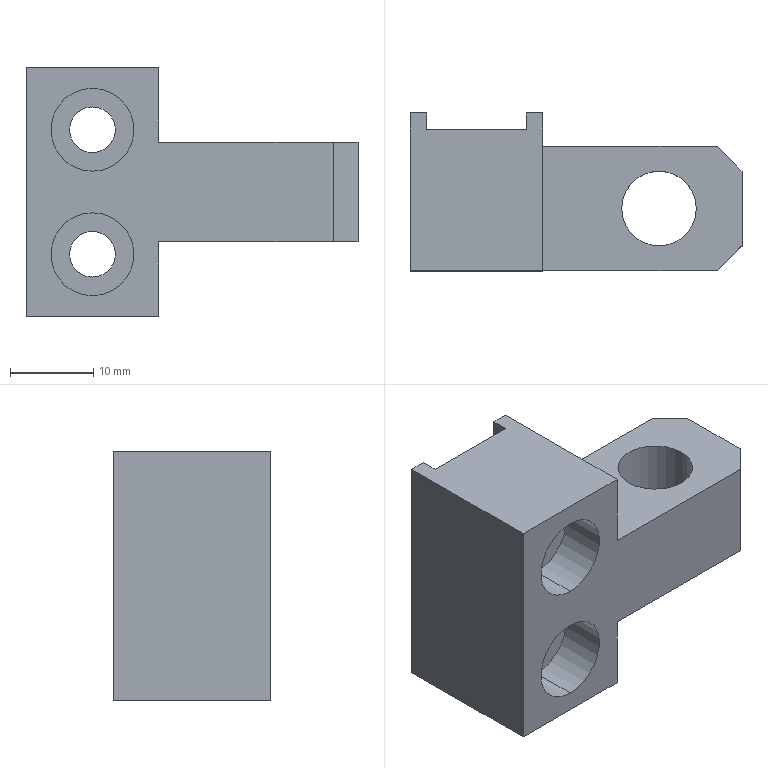Part | STEP file | PN_0025 | 1 solid | 28 faces | box 40 x 19 x 30 mm | volume 10416 mm3 | plane 18 | cylinder 10 | commonest cylinder face diameters 5.5 x4 10 x4 9 x2